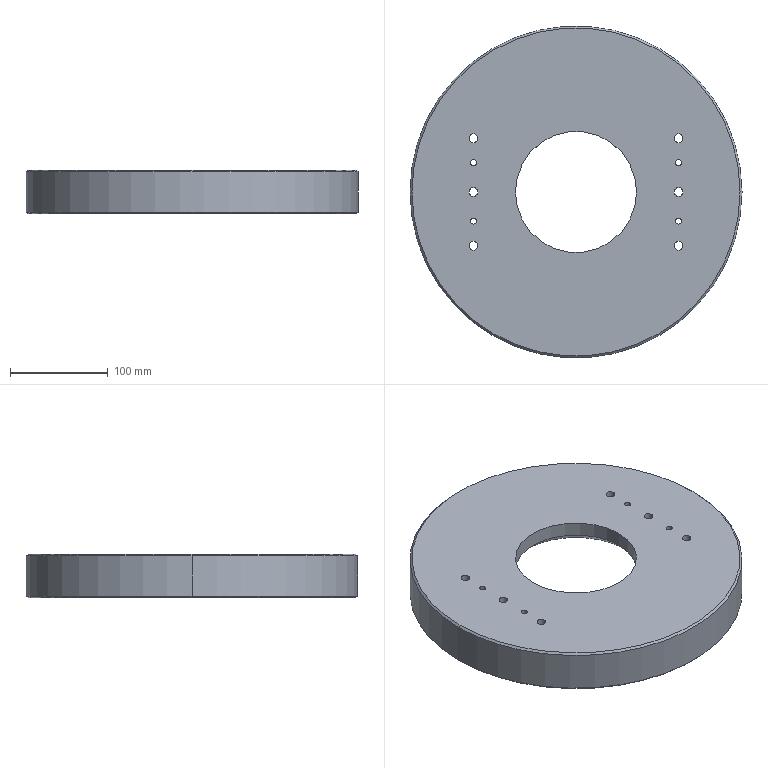CAM job | NX | 3-axis milling, drilling | part box 340 x 340 x 45 mm | stock box 352 x 352 x 49 mm
Tools:
number,name,description,diameter,corner_radius,flute_length,length,flutes
1,D63,Milling Tool-5 Parameters,63.0,0.0,50.0,75.0,2
10,D10,Milling Tool-5 Parameters,10.0,0.0,50.0,75.0,2
11,D10JING,Milling Tool-5 Parameters,10.0,0.0,50.0,75.0,2
7,D6A45,Milling Tool-5 Parameters,6.0,0.0,3.0,3.0,2
18,5.8ZT,Drilling Tool,5.8,0.0,35.0,50.0,2
19,6.0JD,Milling Tool-5 Parameters,6.0,0.0,30.0,30.0,4
9,9.0ZT,Drilling Tool,9.0,0.0,35.0,50.0,2
5,D6R0.5,Milling Tool-5 Parameters,6.0,0.5,50.0,75.0,2
Operations:
program,operation,operation_type,tool,method,geometry_group,spindle_rpm,surface_speed,feed_per_tooth,feed_cut,feed_plunge,cut_length_mm,path_length_mm,cut_time_min,machine_time_min
1-350-48_BLANK_ABGLUE,FLOOR_WALL,VolumeBased25DMillingOperation,D63,METHOD,A,6500.0,1286.0,0.0962,1250.0,100.0,13970.464,14782.413,11.176,11.258
1-350-48_BLANK_ABGLUE,ZLEVEL_PROFILE,ZLevelMilling,D10,METHOD,A,7000.0,219.0,0.2143,3000.0,1000.0,49614.277,49715.677,16.57,16.58
1-350-48_BLANK_ABGLUE,ADAPTIVE_MILLING,CavityMilling,D10,METHOD,A,7000.0,219.0,0.2143,3000.0,1000.0,186711.492,199279.952,64.432,65.689
1-350-48_BLANK_ABGLUE,DRILLING_COPY_1,Operation,D6A45,METHOD,A,3000.0,56.0,0.0333,200.0,0.0,44.0,676.457,0.22,0.2832
1-350-48_BLANK_ABGLUE,DRILLING_COPY_1_COPY_COPY_1,Operation,5.8ZT,METHOD,A,2000.0,18.0,0.03,120.0,0.0,124.97,689.111,1.041,1.098
1-350-48_BLANK_ABGLUE,DRILLING_COPY_1_COPY_COPY_1_COPY,Operation,6.0JD,METHOD,A,1000.0,9.0,0.01,40.0,0.0,114.0,667.171,2.85,2.905
1-350-48_BLANK_ABGLUE,DRILLING_COPY_1_COPY_COPY_1_COPY_1,Operation,9.0ZT,METHOD,A,2000.0,18.0,0.03,120.0,0.0,193.223,958.858,1.61,1.687
1-350-48_BLANK_ABGLUE,FLOOR_WALL_1_COPY_1,VolumeBased25DMillingOperation,D10JING,METHOD,A,7000.0,87.0,0.0714,1000.0,100.0,14553.27,15840.762,14.553,14.723
1-350-48_BLANK_ABGLUE,HOLE_MILLING,CylinderMilling,D10JING,METHOD,A,7000.0,131.0,0.0714,1000.0,100.0,1762.567,2971.65,1.763,1.883
1-350-48_BLANK_ABGLUE,ZLEVEL_PROFILE_COPY_COPY_1_COPY_COPY_2_COPY_1,ZLevelMilling,D6R0.5,METHOD,A,7000.0,131.0,0.2143,3000.0,100.0,55131.48,55983.409,18.377,18.462
1-350-48_BLANK_ABGLUE,ZLEVEL_PROFILE_COPY_COPY_1_COPY_COPY_2_COPY_1_COPY,ZLevelMilling,D6R0.5,METHOD,A,7000.0,131.0,0.2143,3000.0,100.0,59929.477,60040.048,19.977,19.988
1-350-48_BLANK_ABGLUE,CUTTERCOMP11,VolumeBased25DMillingOperation,D10JING,METHOD,A,7000.0,87.0,0.0714,1000.0,100.0,1765.87,2013.31,1.766,1.791
1-350-48_BLANK_ABGLUE,CUTTERCOMP11_COPY,VolumeBased25DMillingOperation,D10JING,METHOD,A,7000.0,87.0,0.0714,1000.0,100.0,365.475,512.475,0.3655,0.3802
1-350-48_BLANK_ABGLUE,ZLEVEL_PROFILE_COPY_1_COPY_COPY_COPY_COPY_2_COPY,ZLevelMilling,D6A45,METHOD,A,7000.0,131.0,0.0714,1000.0,1000.0,2070.697,2215.515,2.071,2.085
1-350-48_BLANK_ABGLUE,ZLEVEL_PROFILE_COPY_1_COPY_COPY_COPY_COPY_2_COPY_COPY,ZLevelMilling,D6A45,METHOD,A,7000.0,131.0,0.0714,1000.0,1000.0,215.435,2558.136,0.2154,0.4497
1-350-48_BLANK_ABGLUE,ZLEVEL_PROFILE_COPY_1,ZLevelMilling,D10JING,METHOD,A,7000.0,219.0,0.0714,1000.0,1000.0,5053.216,5155.966,5.053,5.064
2-350-48_BLANK_ABGLUE,FLOOR_WALL_COPY,VolumeBased25DMillingOperation,D63,METHOD,B,6500.0,1286.0,0.0962,1250.0,100.0,4173.682,4227.682,3.339,3.344
2-350-48_BLANK_ABGLUE,ZLEVEL_PROFILE_COPY_1_COPY_COPY_COPY_COPY_2_COPY_COPY_1,ZLevelMilling,D6A45,METHOD,B,7000.0,131.0,0.0714,1000.0,1000.0,1074.611,1139.611,1.075,1.081
2-350-48_BLANK_ABGLUE,ZLEVEL_PROFILE_COPY_1_COPY_COPY_COPY_COPY_2_COPY_COPY_1_COPY,ZLevelMilling,D6A45,METHOD,B,7000.0,131.0,0.0714,1000.0,1000.0,377.466,442.466,0.3775,0.384